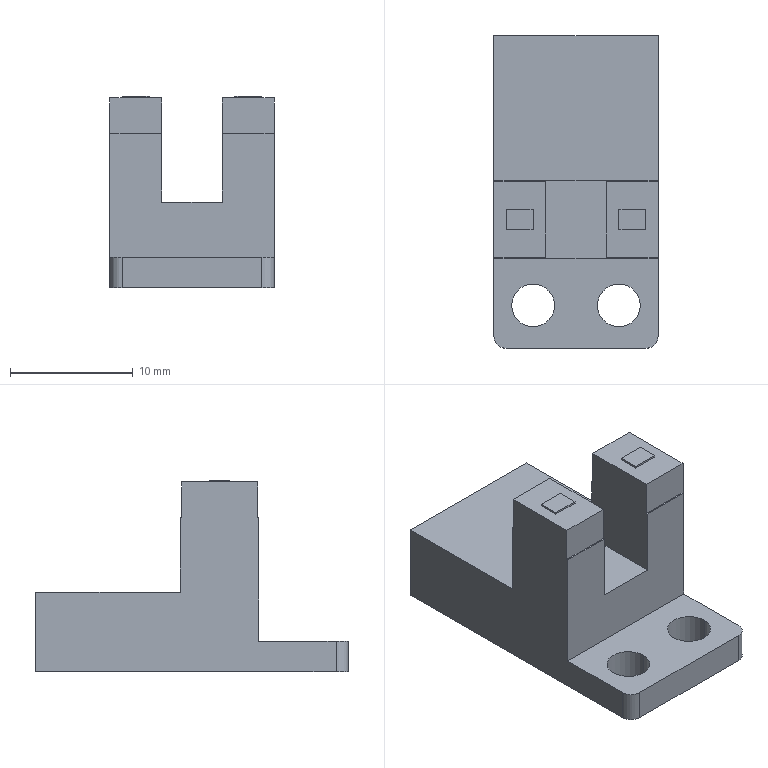Part | SolidWorks | features BaseBody 1 | 1 solid | 38 faces | box 13.4 x 25.5 x 15.65 mm | volume 2278 mm3 | plane 32 | cylinder 6 | commonest cylinder face diameters 3.5 x4 2 x2
STEP:
#1=CARTESIAN_POINT('',(304.797,206.806,-399.345));
#2=VERTEX_POINT('',#1);
#3=CARTESIAN_POINT('',(301.297,206.806,-399.345));
#4=VERTEX_POINT('',#3);
#5=CARTESIAN_POINT('',(303.047,206.806,-399.345));
#6=DIRECTION('',(0.,0.,-1.));
#7=DIRECTION('',(-1.,0.,0.));
#8=AXIS2_PLACEMENT_3D('',#5,#6,#7);
#9=CIRCLE('',#8,1.75);
#10=EDGE_CURVE('',#2,#4,#9,.T.);
#11=ORIENTED_EDGE('',*,*,#10,.F.);
#12=CARTESIAN_POINT('',(304.797,206.806,-401.845));
#13=VERTEX_POINT('',#12);
#14=CARTESIAN_POINT('',(304.797,206.806,-344.345));
#15=DIRECTION('',(0.,0.,-1.));
#16=VECTOR('',#15,1000.);
#17=LINE('',#14,#16);
#18=EDGE_CURVE('',#2,#13,#17,.T.);
#19=ORIENTED_EDGE('',*,*,#18,.T.);
#20=CARTESIAN_POINT('',(301.297,206.806,-401.845));
#21=VERTEX_POINT('',#20);
#22=CARTESIAN_POINT('',(303.047,206.806,-401.845));
#23=DIRECTION('',(0.,0.,-1.));
#24=DIRECTION('',(-1.,0.,0.));
#25=AXIS2_PLACEMENT_3D('',#22,#23,#24);
#26=CIRCLE('',#25,1.75);
#27=EDGE_CURVE('',#13,#21,#26,.T.);
#28=ORIENTED_EDGE('',*,*,#27,.T.);
#29=CARTESIAN_POINT('',(301.297,206.806,-344.345));
#30=DIRECTION('',(0.,0.,-1.));
#31=VECTOR('',#30,1000.);
#32=LINE('',#29,#31);
#33=EDGE_CURVE('',#4,#21,#32,.T.);
#34=ORIENTED_EDGE('',*,*,#33,.F.);
#35=EDGE_LOOP('',(#11,#19,#28,#34));
#36=FACE_OUTER_BOUND('',#35,.T.);
#37=CARTESIAN_POINT('',(303.047,206.806,-344.345));
#38=DIRECTION('',(0.,0.,-1.));
#39=DIRECTION('',(-1.,0.,0.));
#40=AXIS2_PLACEMENT_3D('',#37,#38,#39);
#41=CYLINDRICAL_SURFACE('',#40,1.75);
#42=ADVANCED_FACE('',(#36),#41,.F.);
#43=CARTESIAN_POINT('',(297.797,206.806,-399.345));
#44=VERTEX_POINT('',#43);
#45=CARTESIAN_POINT('',(294.297,206.806,-399.345));
#46=VERTEX_POINT('',#45);
#47=CARTESIAN_POINT('',(296.047,206.806,-399.345));
#48=DIRECTION('',(0.,0.,-1.));
#49=DIRECTION('',(-1.,0.,0.));
#50=AXIS2_PLACEMENT_3D('',#47,#48,#49);
#51=CIRCLE('',#50,1.75);
#52=EDGE_CURVE('',#44,#46,#51,.T.);
#53=ORIENTED_EDGE('',*,*,#52,.F.);
#54=CARTESIAN_POINT('',(297.797,206.806,-401.845));
#55=VERTEX_POINT('',#54);
#56=CARTESIAN_POINT('',(297.797,206.806,-344.345));
#57=DIRECTION('',(0.,0.,-1.));
#58=VECTOR('',#57,1000.);
#59=LINE('',#56,#58);
#60=EDGE_CURVE('',#44,#55,#59,.T.);
#61=ORIENTED_EDGE('',*,*,#60,.T.);
#62=CARTESIAN_POINT('',(294.297,206.806,-401.845));
#63=VERTEX_POINT('',#62);
#64=CARTESIAN_POINT('',(296.047,206.806,-401.845));
#65=DIRECTION('',(0.,0.,-1.));
#66=DIRECTION('',(-1.,0.,0.));
#67=AXIS2_PLACEMENT_3D('',#64,#65,#66);
#68=CIRCLE('',#67,1.75);
#69=EDGE_CURVE('',#55,#63,#68,.T.);
#70=ORIENTED_EDGE('',*,*,#69,.T.);
#71=CARTESIAN_POINT('',(294.297,206.806,-344.345));
#72=DIRECTION('',(0.,0.,-1.));
#73=VECTOR('',#72,1000.);
#74=LINE('',#71,#73);
#75=EDGE_CURVE('',#46,#63,#74,.T.);
#76=ORIENTED_EDGE('',*,*,#75,.F.);
#77=EDGE_LOOP('',(#53,#61,#70,#76));
#78=FACE_OUTER_BOUND('',#77,.T.);
#79=CARTESIAN_POINT('',(296.047,206.806,-344.345));
#80=DIRECTION('',(0.,0.,-1.));
#81=DIRECTION('',(-1.,0.,0.));
#82=AXIS2_PLACEMENT_3D('',#79,#80,#81);
#83=CYLINDRICAL_SURFACE('',#82,1.75);
#84=ADVANCED_FACE('',(#78),#83,.F.);
#85=CARTESIAN_POINT('',(303.047,206.806,-401.845));
#86=DIRECTION('',(0.,0.,-1.));
#87=DIRECTION('',(-1.,0.,0.));
#88=AXIS2_PLACEMENT_3D('',#85,#86,#87);
#89=CIRCLE('',#88,1.75);
#90=EDGE_CURVE('',#21,#13,#89,.T.);
#91=ORIENTED_EDGE('',*,*,#90,.F.);
#92=ORIENTED_EDGE('',*,*,#27,.F.);
#93=EDGE_LOOP('',(#91,#92));
#94=FACE_BOUND('',#93,.T.);
#95=CARTESIAN_POINT('',(296.047,206.806,-401.845));
#96=DIRECTION('',(0.,0.,-1.));
#97=DIRECTION('',(-1.,0.,0.));
#98=AXIS2_PLACEMENT_3D('',#95,#96,#97);
#99=CIRCLE('',#98,1.75);
#100=EDGE_CURVE('',#63,#55,#99,.T.);
#101=ORIENTED_EDGE('',*,*,#100,.F.);
#102=ORIENTED_EDGE('',*,*,#69,.F.);
#103=EDGE_LOOP('',(#101,#102));
#104=FACE_BOUND('',#103,.T.);
#105=CARTESIAN_POINT('',(292.847,228.806,-401.845));
#106=VERTEX_POINT('',#105);
#107=CARTESIAN_POINT('',(292.847,204.306,-401.845));
#108=VERTEX_POINT('',#107);
#109=CARTESIAN_POINT('',(292.847,228.806,-401.845));
#110=DIRECTION('',(0.,-1.,0.));
#111=VECTOR('',#110,1000.);
#112=LINE('',#109,#111);
#113=EDGE_CURVE('',#106,#108,#112,.T.);
#114=ORIENTED_EDGE('',*,*,#113,.F.);
#115=CARTESIAN_POINT('',(306.247,228.806,-401.845));
#116=VERTEX_POINT('',#115);
#117=CARTESIAN_POINT('',(306.247,228.806,-401.845));
#118=DIRECTION('',(-1.,0.,0.));
#119=VECTOR('',#118,1000.);
#120=LINE('',#117,#119);
#121=EDGE_CURVE('',#116,#106,#120,.T.);
#122=ORIENTED_EDGE('',*,*,#121,.F.);
#123=CARTESIAN_POINT('',(306.247,204.306,-401.845));
#124=VERTEX_POINT('',#123);
#125=CARTESIAN_POINT('',(306.247,228.806,-401.845));
#126=DIRECTION('',(0.,1.,0.));
#127=VECTOR('',#126,1000.);
#128=LINE('',#125,#127);
#129=EDGE_CURVE('',#124,#116,#128,.T.);
#130=ORIENTED_EDGE('',*,*,#129,.F.);
#131=CARTESIAN_POINT('',(305.247,203.306,-401.845));
#132=VERTEX_POINT('',#131);
#133=CARTESIAN_POINT('',(305.247,204.306,-401.845));
#134=DIRECTION('',(0.,0.,1.));
#135=DIRECTION('',(-1.,0.,0.));
#136=AXIS2_PLACEMENT_3D('',#133,#134,#135);
#137=CIRCLE('',#136,1.);
#138=EDGE_CURVE('',#132,#124,#137,.T.);
#139=ORIENTED_EDGE('',*,*,#138,.F.);
#140=CARTESIAN_POINT('',(293.847,203.306,-401.845));
#141=VERTEX_POINT('',#140);
#142=CARTESIAN_POINT('',(306.247,203.306,-401.845));
#143=DIRECTION('',(1.,0.,0.));
#144=VECTOR('',#143,1000.);
#145=LINE('',#142,#144);
#146=EDGE_CURVE('',#141,#132,#145,.T.);
#147=ORIENTED_EDGE('',*,*,#146,.F.);
#148=CARTESIAN_POINT('',(293.847,204.306,-401.845));
#149=DIRECTION('',(0.,0.,1.));
#150=DIRECTION('',(1.,0.,0.));
#151=AXIS2_PLACEMENT_3D('',#148,#149,#150);
#152=CIRCLE('',#151,1.);
#153=EDGE_CURVE('',#108,#141,#152,.T.);
#154=ORIENTED_EDGE('',*,*,#153,.F.);
#155=EDGE_LOOP('',(#114,#122,#130,#139,#147,#154));
#156=FACE_OUTER_BOUND('',#155,.T.);
#157=CARTESIAN_POINT('',(306.247,228.806,-401.845));
#158=DIRECTION('',(0.,0.,1.));
#159=DIRECTION('',(1.,0.,0.));
#160=AXIS2_PLACEMENT_3D('',#157,#158,#159);
#161=PLANE('',#160);
#162=ADVANCED_FACE('',(#94,#104,#156),#161,.F.);
#163=ORIENTED_EDGE('',*,*,#18,.F.);
#164=CARTESIAN_POINT('',(303.047,206.806,-399.345));
#165=DIRECTION('',(0.,0.,-1.));
#166=DIRECTION('',(-1.,0.,0.));
#167=AXIS2_PLACEMENT_3D('',#164,#165,#166);
#168=CIRCLE('',#167,1.75);
#169=EDGE_CURVE('',#4,#2,#168,.T.);
#170=ORIENTED_EDGE('',*,*,#169,.F.);
#171=ORIENTED_EDGE('',*,*,#33,.T.);
#172=ORIENTED_EDGE('',*,*,#90,.T.);
#173=EDGE_LOOP('',(#163,#170,#171,#172));
#174=FACE_OUTER_BOUND('',#173,.T.);
#175=CARTESIAN_POINT('',(303.047,206.806,-344.345));
#176=DIRECTION('',(0.,0.,-1.));
#177=DIRECTION('',(-1.,0.,0.));
#178=AXIS2_PLACEMENT_3D('',#175,#176,#177);
#179=CYLINDRICAL_SURFACE('',#178,1.75);
#180=ADVANCED_FACE('',(#174),#179,.F.);
#181=ORIENTED_EDGE('',*,*,#60,.F.);
#182=CARTESIAN_POINT('',(296.047,206.806,-399.345));
#183=DIRECTION('',(0.,0.,-1.));
#184=DIRECTION('',(-1.,0.,0.));
#185=AXIS2_PLACEMENT_3D('',#182,#183,#184);
#186=CIRCLE('',#185,1.75);
#187=EDGE_CURVE('',#46,#44,#186,.T.);
#188=ORIENTED_EDGE('',*,*,#187,.F.);
#189=ORIENTED_EDGE('',*,*,#75,.T.);
#190=ORIENTED_EDGE('',*,*,#100,.T.);
#191=EDGE_LOOP('',(#181,#188,#189,#190));
#192=FACE_OUTER_BOUND('',#191,.T.);
#193=CARTESIAN_POINT('',(296.047,206.806,-344.345));
#194=DIRECTION('',(0.,0.,-1.));
#195=DIRECTION('',(-1.,0.,0.));
#196=AXIS2_PLACEMENT_3D('',#193,#194,#195);
#197=CYLINDRICAL_SURFACE('',#196,1.75);
#198=ADVANCED_FACE('',(#192),#197,.F.);
#199=CARTESIAN_POINT('',(292.847,204.306,-399.345));
#200=VERTEX_POINT('',#199);
#201=CARTESIAN_POINT('',(292.847,204.306,-401.845));
#202=DIRECTION('',(0.,0.,-1.));
#203=VECTOR('',#202,1000.);
#204=LINE('',#201,#203);
#205=EDGE_CURVE('',#200,#108,#204,.T.);
#206=ORIENTED_EDGE('',*,*,#205,.T.);
#207=ORIENTED_EDGE('',*,*,#153,.T.);
#208=CARTESIAN_POINT('',(293.847,203.306,-399.345));
#209=VERTEX_POINT('',#208);
#210=CARTESIAN_POINT('',(293.847,203.306,-401.845));
#211=DIRECTION('',(0.,0.,1.));
#212=VECTOR('',#211,1000.);
#213=LINE('',#210,#212);
#214=EDGE_CURVE('',#141,#209,#213,.T.);
#215=ORIENTED_EDGE('',*,*,#214,.T.);
#216=CARTESIAN_POINT('',(293.847,204.306,-399.345));
#217=DIRECTION('',(0.,0.,-1.));
#218=DIRECTION('',(1.,0.,0.));
#219=AXIS2_PLACEMENT_3D('',#216,#217,#218);
#220=CIRCLE('',#219,1.);
#221=EDGE_CURVE('',#209,#200,#220,.T.);
#222=ORIENTED_EDGE('',*,*,#221,.T.);
#223=EDGE_LOOP('',(#206,#207,#215,#222));
#224=FACE_OUTER_BOUND('',#223,.T.);
#225=CARTESIAN_POINT('',(293.847,204.306,-401.845));
#226=DIRECTION('',(0.,0.,1.));
#227=DIRECTION('',(1.,0.,0.));
#228=AXIS2_PLACEMENT_3D('',#225,#226,#227);
#229=CYLINDRICAL_SURFACE('',#228,1.);
#230=ADVANCED_FACE('',(#224),#229,.T.);
#231=CARTESIAN_POINT('',(292.847,210.606,-399.345));
#232=VERTEX_POINT('',#231);
#233=CARTESIAN_POINT('',(292.847,228.806,-399.345));
#234=DIRECTION('',(0.,-1.,0.));
#235=VECTOR('',#234,1000.);
#236=LINE('',#233,#235);
#237=EDGE_CURVE('',#232,#200,#236,.T.);
#238=ORIENTED_EDGE('',*,*,#237,.F.);
#239=CARTESIAN_POINT('',(292.847,210.606,-389.245));
#240=VERTEX_POINT('',#239);
#241=CARTESIAN_POINT('',(292.847,210.606,-401.845));
#242=DIRECTION('',(0.,0.,-1.));
#243=VECTOR('',#242,1000.);
#244=LINE('',#241,#243);
#245=EDGE_CURVE('',#240,#232,#244,.T.);
#246=ORIENTED_EDGE('',*,*,#245,.F.);
#247=CARTESIAN_POINT('',(292.847,210.706,-389.245));
#248=VERTEX_POINT('',#247);
#249=CARTESIAN_POINT('',(292.847,228.806,-389.245));
#250=DIRECTION('',(0.,-1.,0.));
#251=VECTOR('',#250,1000.);
#252=LINE('',#249,#251);
#253=EDGE_CURVE('',#248,#240,#252,.T.);
#254=ORIENTED_EDGE('',*,*,#253,.F.);
#255=CARTESIAN_POINT('',(292.847,210.706,-386.345));
#256=VERTEX_POINT('',#255);
#257=CARTESIAN_POINT('',(292.847,210.706,-401.845));
#258=DIRECTION('',(0.,0.,-1.));
#259=VECTOR('',#258,1000.);
#260=LINE('',#257,#259);
#261=EDGE_CURVE('',#256,#248,#260,.T.);
#262=ORIENTED_EDGE('',*,*,#261,.F.);
#263=CARTESIAN_POINT('',(292.847,216.906,-386.345));
#264=VERTEX_POINT('',#263);
#265=CARTESIAN_POINT('',(292.847,228.806,-386.345));
#266=DIRECTION('',(0.,-1.,0.));
#267=VECTOR('',#266,1000.);
#268=LINE('',#265,#267);
#269=EDGE_CURVE('',#264,#256,#268,.T.);
#270=ORIENTED_EDGE('',*,*,#269,.F.);
#271=CARTESIAN_POINT('',(292.847,216.906,-389.245));
#272=VERTEX_POINT('',#271);
#273=CARTESIAN_POINT('',(292.847,216.906,-401.845));
#274=DIRECTION('',(0.,0.,1.));
#275=VECTOR('',#274,1000.);
#276=LINE('',#273,#275);
#277=EDGE_CURVE('',#272,#264,#276,.T.);
#278=ORIENTED_EDGE('',*,*,#277,.F.);
#279=CARTESIAN_POINT('',(292.847,217.006,-389.245));
#280=VERTEX_POINT('',#279);
#281=CARTESIAN_POINT('',(292.847,228.806,-389.245));
#282=DIRECTION('',(0.,-1.,0.));
#283=VECTOR('',#282,1000.);
#284=LINE('',#281,#283);
#285=EDGE_CURVE('',#280,#272,#284,.T.);
#286=ORIENTED_EDGE('',*,*,#285,.F.);
#287=CARTESIAN_POINT('',(292.847,217.006,-395.345));
#288=VERTEX_POINT('',#287);
#289=CARTESIAN_POINT('',(292.847,217.006,-401.845));
#290=DIRECTION('',(0.,0.,1.));
#291=VECTOR('',#290,1000.);
#292=LINE('',#289,#291);
#293=EDGE_CURVE('',#288,#280,#292,.T.);
#294=ORIENTED_EDGE('',*,*,#293,.F.);
#295=CARTESIAN_POINT('',(292.847,228.806,-395.345));
#296=VERTEX_POINT('',#295);
#297=CARTESIAN_POINT('',(292.847,228.806,-395.345));
#298=DIRECTION('',(0.,-1.,0.));
#299=VECTOR('',#298,1000.);
#300=LINE('',#297,#299);
#301=EDGE_CURVE('',#296,#288,#300,.T.);
#302=ORIENTED_EDGE('',*,*,#301,.F.);
#303=CARTESIAN_POINT('',(292.847,228.806,-401.845));
#304=DIRECTION('',(0.,0.,1.));
#305=VECTOR('',#304,1000.);
#306=LINE('',#303,#305);
#307=EDGE_CURVE('',#106,#296,#306,.T.);
#308=ORIENTED_EDGE('',*,*,#307,.F.);
#309=ORIENTED_EDGE('',*,*,#113,.T.);
#310=ORIENTED_EDGE('',*,*,#205,.F.);
#311=EDGE_LOOP('',(#238,#246,#254,#262,#270,#278,#286,#294,#302,#308,#309,#310));
#312=FACE_OUTER_BOUND('',#311,.T.);
#313=CARTESIAN_POINT('',(292.847,228.806,-401.845));
#314=DIRECTION('',(1.,0.,0.));
#315=DIRECTION('',(0.,0.,-1.));
#316=AXIS2_PLACEMENT_3D('',#313,#314,#315);
#317=PLANE('',#316);
#318=ADVANCED_FACE('',(#312),#317,.F.);
#319=ORIENTED_EDGE('',*,*,#307,.T.);
#320=CARTESIAN_POINT('',(306.247,228.806,-395.345));
#321=VERTEX_POINT('',#320);
#322=CARTESIAN_POINT('',(357.247,228.806,-395.345));
#323=DIRECTION('',(1.,0.,0.));
#324=VECTOR('',#323,1000.);
#325=LINE('',#322,#324);
#326=EDGE_CURVE('',#296,#321,#325,.T.);
#327=ORIENTED_EDGE('',*,*,#326,.T.);
#328=CARTESIAN_POINT('',(306.247,228.806,-444.345));
#329=DIRECTION('',(0.,0.,-1.));
#330=VECTOR('',#329,1000.);
#331=LINE('',#328,#330);
#332=EDGE_CURVE('',#321,#116,#331,.T.);
#333=ORIENTED_EDGE('',*,*,#332,.T.);
#334=ORIENTED_EDGE('',*,*,#121,.T.);
#335=EDGE_LOOP('',(#319,#327,#333,#334));
#336=FACE_OUTER_BOUND('',#335,.T.);
#337=CARTESIAN_POINT('',(357.247,228.806,-444.345));
#338=DIRECTION('',(0.,1.,0.));
#339=DIRECTION('',(0.,0.,1.));
#340=AXIS2_PLACEMENT_3D('',#337,#338,#339);
#341=PLANE('',#340);
#342=ADVANCED_FACE('',(#336),#341,.T.);
#343=ORIENTED_EDGE('',*,*,#129,.T.);
#344=ORIENTED_EDGE('',*,*,#332,.F.);
#345=CARTESIAN_POINT('',(306.247,217.006,-395.345));
#346=VERTEX_POINT('',#345);
#347=CARTESIAN_POINT('',(306.247,228.806,-395.345));
#348=DIRECTION('',(0.,1.,0.));
#349=VECTOR('',#348,1000.);
#350=LINE('',#347,#349);
#351=EDGE_CURVE('',#346,#321,#350,.T.);
#352=ORIENTED_EDGE('',*,*,#351,.F.);
#353=CARTESIAN_POINT('',(306.247,217.006,-389.245));
#354=VERTEX_POINT('',#353);
#355=CARTESIAN_POINT('',(306.247,217.006,-386.345));
#356=DIRECTION('',(0.,0.,-1.));
#357=VECTOR('',#356,1000.);
#358=LINE('',#355,#357);
#359=EDGE_CURVE('',#354,#346,#358,.T.);
#360=ORIENTED_EDGE('',*,*,#359,.F.);
#361=CARTESIAN_POINT('',(306.247,216.906,-389.245));
#362=VERTEX_POINT('',#361);
#363=CARTESIAN_POINT('',(306.247,228.806,-389.245));
#364=DIRECTION('',(0.,1.,0.));
#365=VECTOR('',#364,1000.);
#366=LINE('',#363,#365);
#367=EDGE_CURVE('',#362,#354,#366,.T.);
#368=ORIENTED_EDGE('',*,*,#367,.F.);
#369=CARTESIAN_POINT('',(306.247,216.906,-386.345));
#370=VERTEX_POINT('',#369);
#371=CARTESIAN_POINT('',(306.247,216.906,-386.345));
#372=DIRECTION('',(0.,0.,-1.));
#373=VECTOR('',#372,1000.);
#374=LINE('',#371,#373);
#375=EDGE_CURVE('',#370,#362,#374,.T.);
#376=ORIENTED_EDGE('',*,*,#375,.F.);
#377=CARTESIAN_POINT('',(306.247,210.706,-386.345));
#378=VERTEX_POINT('',#377);
#379=CARTESIAN_POINT('',(306.247,228.806,-386.345));
#380=DIRECTION('',(0.,1.,0.));
#381=VECTOR('',#380,1000.);
#382=LINE('',#379,#381);
#383=EDGE_CURVE('',#378,#370,#382,.T.);
#384=ORIENTED_EDGE('',*,*,#383,.F.);
#385=CARTESIAN_POINT('',(306.247,210.706,-389.245));
#386=VERTEX_POINT('',#385);
#387=CARTESIAN_POINT('',(306.247,210.706,-386.345));
#388=DIRECTION('',(0.,0.,1.));
#389=VECTOR('',#388,1000.);
#390=LINE('',#387,#389);
#391=EDGE_CURVE('',#386,#378,#390,.T.);
#392=ORIENTED_EDGE('',*,*,#391,.F.);
#393=CARTESIAN_POINT('',(306.247,210.606,-389.245));
#394=VERTEX_POINT('',#393);
#395=CARTESIAN_POINT('',(306.247,228.806,-389.245));
#396=DIRECTION('',(0.,1.,0.));
#397=VECTOR('',#396,1000.);
#398=LINE('',#395,#397);
#399=EDGE_CURVE('',#394,#386,#398,.T.);
#400=ORIENTED_EDGE('',*,*,#399,.F.);
#401=CARTESIAN_POINT('',(306.247,210.606,-399.345));
#402=VERTEX_POINT('',#401);
#403=CARTESIAN_POINT('',(306.247,210.606,-386.345));
#404=DIRECTION('',(0.,0.,1.));
#405=VECTOR('',#404,1000.);
#406=LINE('',#403,#405);
#407=EDGE_CURVE('',#402,#394,#406,.T.);
#408=ORIENTED_EDGE('',*,*,#407,.F.);
#409=CARTESIAN_POINT('',(306.247,204.306,-399.345));
#410=VERTEX_POINT('',#409);
#411=CARTESIAN_POINT('',(306.247,228.806,-399.345));
#412=DIRECTION('',(0.,1.,0.));
#413=VECTOR('',#412,1000.);
#414=LINE('',#411,#413);
#415=EDGE_CURVE('',#410,#402,#414,.T.);
#416=ORIENTED_EDGE('',*,*,#415,.F.);
#417=CARTESIAN_POINT('',(306.247,204.306,-386.345));
#418=DIRECTION('',(0.,0.,1.));
#419=VECTOR('',#418,1000.);
#420=LINE('',#417,#419);
#421=EDGE_CURVE('',#124,#410,#420,.T.);
#422=ORIENTED_EDGE('',*,*,#421,.F.);
#423=EDGE_LOOP('',(#343,#344,#352,#360,#368,#376,#384,#392,#400,#408,#416,#422));
#424=FACE_OUTER_BOUND('',#423,.T.);
#425=CARTESIAN_POINT('',(306.247,228.806,-386.345));
#426=DIRECTION('',(-1.,0.,0.));
#427=DIRECTION('',(0.,0.,1.));
#428=AXIS2_PLACEMENT_3D('',#425,#426,#427);
#429=PLANE('',#428);
#430=ADVANCED_FACE('',(#424),#429,.F.);
#431=ORIENTED_EDGE('',*,*,#421,.T.);
#432=CARTESIAN_POINT('',(305.247,203.306,-399.345));
#433=VERTEX_POINT('',#432);
#434=CARTESIAN_POINT('',(305.247,204.306,-399.345));
#435=DIRECTION('',(0.,0.,-1.));
#436=DIRECTION('',(-1.,0.,0.));
#437=AXIS2_PLACEMENT_3D('',#434,#435,#436);
#438=CIRCLE('',#437,1.);
#439=EDGE_CURVE('',#410,#433,#438,.T.);
#440=ORIENTED_EDGE('',*,*,#439,.T.);
#441=CARTESIAN_POINT('',(305.247,203.306,-386.345));
#442=DIRECTION('',(0.,0.,-1.));
#443=VECTOR('',#442,1000.);
#444=LINE('',#441,#443);
#445=EDGE_CURVE('',#433,#132,#444,.T.);
#446=ORIENTED_EDGE('',*,*,#445,.T.);
#447=ORIENTED_EDGE('',*,*,#138,.T.);
#448=EDGE_LOOP('',(#431,#440,#446,#447));
#449=FACE_OUTER_BOUND('',#448,.T.);
#450=CARTESIAN_POINT('',(305.247,204.306,-386.345));
#451=DIRECTION('',(0.,0.,-1.));
#452=DIRECTION('',(-1.,0.,0.));
#453=AXIS2_PLACEMENT_3D('',#450,#451,#452);
#454=CYLINDRICAL_SURFACE('',#453,1.);
#455=ADVANCED_FACE('',(#449),#454,.T.);
#456=ORIENTED_EDGE('',*,*,#146,.T.);
#457=ORIENTED_EDGE('',*,*,#445,.F.);
#458=CARTESIAN_POINT('',(357.247,203.306,-399.345));
#459=DIRECTION('',(1.,0.,0.));
#460=VECTOR('',#459,1000.);
#461=LINE('',#458,#460);
#462=EDGE_CURVE('',#209,#433,#461,.T.);
#463=ORIENTED_EDGE('',*,*,#462,.F.);
#464=ORIENTED_EDGE('',*,*,#214,.F.);
#465=EDGE_LOOP('',(#456,#457,#463,#464));
#466=FACE_OUTER_BOUND('',#465,.T.);
#467=CARTESIAN_POINT('',(357.247,203.306,-444.345));
#468=DIRECTION('',(0.,1.,0.));
#469=DIRECTION('',(0.,0.,1.));
#470=AXIS2_PLACEMENT_3D('',#467,#468,#469);
#471=PLANE('',#470);
#472=ADVANCED_FACE('',(#466),#471,.F.);
#473=ORIENTED_EDGE('',*,*,#169,.T.);
#474=ORIENTED_EDGE('',*,*,#10,.T.);
#475=EDGE_LOOP('',(#473,#474));
#476=FACE_BOUND('',#475,.T.);
#477=ORIENTED_EDGE('',*,*,#187,.T.);
#478=ORIENTED_EDGE('',*,*,#52,.T.);
#479=EDGE_LOOP('',(#477,#478));
#480=FACE_BOUND('',#479,.T.);
#481=ORIENTED_EDGE('',*,*,#462,.T.);
#482=ORIENTED_EDGE('',*,*,#439,.F.);
#483=ORIENTED_EDGE('',*,*,#415,.T.);
#484=CARTESIAN_POINT('',(257.247,210.606,-399.345));
#485=DIRECTION('',(1.,0.,0.));
#486=VECTOR('',#485,1000.);
#487=LINE('',#484,#486);
#488=EDGE_CURVE('',#232,#402,#487,.T.);
#489=ORIENTED_EDGE('',*,*,#488,.F.);
#490=ORIENTED_EDGE('',*,*,#237,.T.);
#491=ORIENTED_EDGE('',*,*,#221,.F.);
#492=EDGE_LOOP('',(#481,#482,#483,#489,#490,#491));
#493=FACE_OUTER_BOUND('',#492,.T.);
#494=CARTESIAN_POINT('',(257.247,203.306,-399.345));
#495=DIRECTION('',(0.,0.,-1.));
#496=DIRECTION('',(-1.,0.,0.));
#497=AXIS2_PLACEMENT_3D('',#494,#495,#496);
#498=PLANE('',#497);
#499=ADVANCED_FACE('',(#476,#480,#493),#498,.F.);
#500=CARTESIAN_POINT('',(297.063,210.606,-394.845));
#501=VERTEX_POINT('',#500);
#502=CARTESIAN_POINT('',(302.031,210.606,-394.845));
#503=VERTEX_POINT('',#502);
#504=CARTESIAN_POINT('',(257.247,210.606,-394.845));
#505=DIRECTION('',(1.,0.,0.));
#506=VECTOR('',#505,1000.);
#507=LINE('',#504,#506);
#508=EDGE_CURVE('',#501,#503,#507,.T.);
#509=ORIENTED_EDGE('',*,*,#508,.F.);
#510=CARTESIAN_POINT('',(297.063,210.606,-389.245));
#511=VERTEX_POINT('',#510);
#512=CARTESIAN_POINT('',(297.063,210.606,-399.345));
#513=DIRECTION('',(0.,0.,-1.));
#514=VECTOR('',#513,1000.);
#515=LINE('',#512,#514);
#516=EDGE_CURVE('',#511,#501,#515,.T.);
#517=ORIENTED_EDGE('',*,*,#516,.F.);
#518=CARTESIAN_POINT('',(257.247,210.606,-389.245));
#519=DIRECTION('',(1.,0.,0.));
#520=VECTOR('',#519,1000.);
#521=LINE('',#518,#520);
#522=EDGE_CURVE('',#240,#511,#521,.T.);
#523=ORIENTED_EDGE('',*,*,#522,.F.);
#524=ORIENTED_EDGE('',*,*,#245,.T.);
#525=ORIENTED_EDGE('',*,*,#488,.T.);
#526=ORIENTED_EDGE('',*,*,#407,.T.);
#527=CARTESIAN_POINT('',(302.031,210.606,-389.245));
#528=VERTEX_POINT('',#527);
#529=CARTESIAN_POINT('',(257.247,210.606,-389.245));
#530=DIRECTION('',(1.,0.,0.));
#531=VECTOR('',#530,1000.);
#532=LINE('',#529,#531);
#533=EDGE_CURVE('',#528,#394,#532,.T.);
#534=ORIENTED_EDGE('',*,*,#533,.F.);
#535=CARTESIAN_POINT('',(302.031,210.606,-399.345));
#536=DIRECTION('',(0.,0.,1.));
#537=VECTOR('',#536,1000.);
#538=LINE('',#535,#537);
#539=EDGE_CURVE('',#503,#528,#538,.T.);
#540=ORIENTED_EDGE('',*,*,#539,.F.);
#541=EDGE_LOOP('',(#509,#517,#523,#524,#525,#526,#534,#540));
#542=FACE_OUTER_BOUND('',#541,.T.);
#543=CARTESIAN_POINT('',(257.247,210.606,-399.345));
#544=DIRECTION('',(0.,1.,0.));
#545=DIRECTION('',(0.,0.,1.));
#546=AXIS2_PLACEMENT_3D('',#543,#544,#545);
#547=PLANE('',#546);
#548=ADVANCED_FACE('',(#542),#547,.F.);
#549=CARTESIAN_POINT('',(297.063,210.706,-389.245));
#550=VERTEX_POINT('',#549);
#551=CARTESIAN_POINT('',(257.247,210.706,-389.245));
#552=DIRECTION('',(1.,0.,0.));
#553=VECTOR('',#552,1000.);
#554=LINE('',#551,#553);
#555=EDGE_CURVE('',#248,#550,#554,.T.);
#556=ORIENTED_EDGE('',*,*,#555,.F.);
#557=ORIENTED_EDGE('',*,*,#253,.T.);
#558=ORIENTED_EDGE('',*,*,#522,.T.);
#559=CARTESIAN_POINT('',(297.063,210.606,-389.245));
#560=DIRECTION('',(0.,-1.,0.));
#561=VECTOR('',#560,1000.);
#562=LINE('',#559,#561);
#563=EDGE_CURVE('',#550,#511,#562,.T.);
#564=ORIENTED_EDGE('',*,*,#563,.F.);
#565=EDGE_LOOP('',(#556,#557,#558,#564));
#566=FACE_OUTER_BOUND('',#565,.T.);
#567=CARTESIAN_POINT('',(257.247,210.606,-389.245));
#568=DIRECTION('',(0.,0.,-1.));
#569=DIRECTION('',(-1.,0.,0.));
#570=AXIS2_PLACEMENT_3D('',#567,#568,#569);
#571=PLANE('',#570);
#572=ADVANCED_FACE('',(#566),#571,.F.);
#573=CARTESIAN_POINT('',(297.063,210.706,-386.345));
#574=VERTEX_POINT('',#573);
#575=CARTESIAN_POINT('',(257.247,210.706,-386.345));
#576=DIRECTION('',(1.,0.,0.));
#577=VECTOR('',#576,1000.);
#578=LINE('',#575,#577);
#579=EDGE_CURVE('',#256,#574,#578,.T.);
#580=ORIENTED_EDGE('',*,*,#579,.F.);
#581=ORIENTED_EDGE('',*,*,#261,.T.);
#582=ORIENTED_EDGE('',*,*,#555,.T.);
#583=CARTESIAN_POINT('',(297.063,210.706,-389.245));
#584=DIRECTION('',(0.,0.,-1.));
#585=VECTOR('',#584,1000.);
#586=LINE('',#583,#585);
#587=EDGE_CURVE('',#574,#550,#586,.T.);
#588=ORIENTED_EDGE('',*,*,#587,.F.);
#589=EDGE_LOOP('',(#580,#581,#582,#588));
#590=FACE_OUTER_BOUND('',#589,.T.);
#591=CARTESIAN_POINT('',(257.247,210.706,-389.245));
#592=DIRECTION('',(0.,1.,0.));
#593=DIRECTION('',(0.,0.,1.));
#594=AXIS2_PLACEMENT_3D('',#591,#592,#593);
#595=PLANE('',#594);
#596=ADVANCED_FACE('',(#590),#595,.F.);
#597=CARTESIAN_POINT('',(296.047,214.646,-386.345));
#598=VERTEX_POINT('',#597);
#599=CARTESIAN_POINT('',(293.847,214.646,-386.345));
#600=VERTEX_POINT('',#599);
#601=CARTESIAN_POINT('',(296.047,214.646,-386.345));
#602=DIRECTION('',(-1.,0.,0.));
#603=VECTOR('',#602,1000.);
#604=LINE('',#601,#603);
#605=EDGE_CURVE('',#598,#600,#604,.T.);
#606=ORIENTED_EDGE('',*,*,#605,.F.);
#607=CARTESIAN_POINT('',(296.047,212.966,-386.345));
#608=VERTEX_POINT('',#607);
#609=CARTESIAN_POINT('',(296.047,228.806,-386.345));
#610=DIRECTION('',(0.,1.,0.));
#611=VECTOR('',#610,1000.);
#612=LINE('',#609,#611);
#613=EDGE_CURVE('',#608,#598,#612,.T.);
#614=ORIENTED_EDGE('',*,*,#613,.F.);
#615=CARTESIAN_POINT('',(293.847,212.966,-386.345));
#616=VERTEX_POINT('',#615);
#617=CARTESIAN_POINT('',(296.047,212.966,-386.345));
#618=DIRECTION('',(1.,0.,0.));
#619=VECTOR('',#618,1000.);
#620=LINE('',#617,#619);
#621=EDGE_CURVE('',#616,#608,#620,.T.);
#622=ORIENTED_EDGE('',*,*,#621,.F.);
#623=CARTESIAN_POINT('',(293.847,228.806,-386.345));
#624=DIRECTION('',(0.,-1.,0.));
#625=VECTOR('',#624,1000.);
#626=LINE('',#623,#625);
#627=EDGE_CURVE('',#600,#616,#626,.T.);
#628=ORIENTED_EDGE('',*,*,#627,.F.);
#629=EDGE_LOOP('',(#606,#614,#622,#628));
#630=FACE_BOUND('',#629,.T.);
#631=CARTESIAN_POINT('',(297.063,216.906,-386.345));
#632=VERTEX_POINT('',#631);
#633=CARTESIAN_POINT('',(297.063,228.806,-386.345));
#634=DIRECTION('',(0.,-1.,0.));
#635=VECTOR('',#634,1000.);
#636=LINE('',#633,#635);
#637=EDGE_CURVE('',#632,#574,#636,.T.);
#638=ORIENTED_EDGE('',*,*,#637,.F.);
#639=CARTESIAN_POINT('',(296.047,216.906,-386.345));
#640=DIRECTION('',(1.,0.,0.));
#641=VECTOR('',#640,1000.);
#642=LINE('',#639,#641);
#643=EDGE_CURVE('',#264,#632,#642,.T.);
#644=ORIENTED_EDGE('',*,*,#643,.F.);
#645=ORIENTED_EDGE('',*,*,#269,.T.);
#646=ORIENTED_EDGE('',*,*,#579,.T.);
#647=EDGE_LOOP('',(#638,#644,#645,#646));
#648=FACE_OUTER_BOUND('',#647,.T.);
#649=CARTESIAN_POINT('',(296.047,228.806,-386.345));
#650=DIRECTION('',(0.,0.,-1.));
#651=DIRECTION('',(-1.,0.,0.));
#652=AXIS2_PLACEMENT_3D('',#649,#650,#651);
#653=PLANE('',#652);
#654=ADVANCED_FACE('',(#630,#648),#653,.F.);
#655=CARTESIAN_POINT('',(297.063,216.906,-389.245));
#656=VERTEX_POINT('',#655);
#657=CARTESIAN_POINT('',(297.063,216.906,-386.345));
#658=DIRECTION('',(0.,0.,1.));
#659=VECTOR('',#658,1000.);
#660=LINE('',#657,#659);
#661=EDGE_CURVE('',#656,#632,#660,.T.);
#662=ORIENTED_EDGE('',*,*,#661,.F.);
#663=CARTESIAN_POINT('',(257.247,216.906,-389.245));
#664=DIRECTION('',(1.,0.,0.));
#665=VECTOR('',#664,1000.);
#666=LINE('',#663,#665);
#667=EDGE_CURVE('',#272,#656,#666,.T.);
#668=ORIENTED_EDGE('',*,*,#667,.F.);
#669=ORIENTED_EDGE('',*,*,#277,.T.);
#670=ORIENTED_EDGE('',*,*,#643,.T.);
#671=EDGE_LOOP('',(#662,#668,#669,#670));
#672=FACE_OUTER_BOUND('',#671,.T.);
#673=CARTESIAN_POINT('',(257.247,216.906,-386.345));
#674=DIRECTION('',(0.,-1.,0.));
#675=DIRECTION('',(0.,0.,-1.));
#676=AXIS2_PLACEMENT_3D('',#673,#674,#675);
#677=PLANE('',#676);
#678=ADVANCED_FACE('',(#672),#677,.F.);
#679=CARTESIAN_POINT('',(297.063,217.006,-389.245));
#680=VERTEX_POINT('',#679);
#681=CARTESIAN_POINT('',(257.247,217.006,-389.245));
#682=DIRECTION('',(1.,0.,0.));
#683=VECTOR('',#682,1000.);
#684=LINE('',#681,#683);
#685=EDGE_CURVE('',#280,#680,#684,.T.);
#686=ORIENTED_EDGE('',*,*,#685,.F.);
#687=ORIENTED_EDGE('',*,*,#285,.T.);
#688=ORIENTED_EDGE('',*,*,#667,.T.);
#689=CARTESIAN_POINT('',(297.063,216.906,-389.245));
#690=DIRECTION('',(0.,-1.,0.));
#691=VECTOR('',#690,1000.);
#692=LINE('',#689,#691);
#693=EDGE_CURVE('',#680,#656,#692,.T.);
#694=ORIENTED_EDGE('',*,*,#693,.F.);
#695=EDGE_LOOP('',(#686,#687,#688,#694));
#696=FACE_OUTER_BOUND('',#695,.T.);
#697=CARTESIAN_POINT('',(257.247,216.906,-389.245));
#698=DIRECTION('',(0.,0.,-1.));
#699=DIRECTION('',(-1.,0.,0.));
#700=AXIS2_PLACEMENT_3D('',#697,#698,#699);
#701=PLANE('',#700);
#702=ADVANCED_FACE('',(#696),#701,.F.);
#703=ORIENTED_EDGE('',*,*,#685,.T.);
#704=CARTESIAN_POINT('',(297.063,217.006,-394.845));
#705=VERTEX_POINT('',#704);
#706=CARTESIAN_POINT('',(297.063,217.006,-389.245));
#707=DIRECTION('',(0.,0.,1.));
#708=VECTOR('',#707,1000.);
#709=LINE('',#706,#708);
#710=EDGE_CURVE('',#705,#680,#709,.T.);
#711=ORIENTED_EDGE('',*,*,#710,.F.);
#712=CARTESIAN_POINT('',(302.031,217.006,-394.845));
#713=VERTEX_POINT('',#712);
#714=CARTESIAN_POINT('',(257.247,217.006,-394.845));
#715=DIRECTION('',(-1.,0.,0.));
#716=VECTOR('',#715,1000.);
#717=LINE('',#714,#716);
#718=EDGE_CURVE('',#713,#705,#717,.T.);
#719=ORIENTED_EDGE('',*,*,#718,.F.);
#720=CARTESIAN_POINT('',(302.031,217.006,-389.245));
#721=VERTEX_POINT('',#720);
#722=CARTESIAN_POINT('',(302.031,217.006,-389.245));
#723=DIRECTION('',(0.,0.,-1.));
#724=VECTOR('',#723,1000.);
#725=LINE('',#722,#724);
#726=EDGE_CURVE('',#721,#713,#725,.T.);
#727=ORIENTED_EDGE('',*,*,#726,.F.);
#728=CARTESIAN_POINT('',(257.247,217.006,-389.245));
#729=DIRECTION('',(-1.,0.,0.));
#730=VECTOR('',#729,1000.);
#731=LINE('',#728,#730);
#732=EDGE_CURVE('',#354,#721,#731,.T.);
#733=ORIENTED_EDGE('',*,*,#732,.F.);
#734=ORIENTED_EDGE('',*,*,#359,.T.);
#735=CARTESIAN_POINT('',(257.247,217.006,-395.345));
#736=DIRECTION('',(1.,0.,0.));
#737=VECTOR('',#736,1000.);
#738=LINE('',#735,#737);
#739=EDGE_CURVE('',#288,#346,#738,.T.);
#740=ORIENTED_EDGE('',*,*,#739,.F.);
#741=ORIENTED_EDGE('',*,*,#293,.T.);
#742=EDGE_LOOP('',(#703,#711,#719,#727,#733,#734,#740,#741));
#743=FACE_OUTER_BOUND('',#742,.T.);
#744=CARTESIAN_POINT('',(257.247,217.006,-389.245));
#745=DIRECTION('',(0.,-1.,0.));
#746=DIRECTION('',(0.,0.,-1.));
#747=AXIS2_PLACEMENT_3D('',#744,#745,#746);
#748=PLANE('',#747);
#749=ADVANCED_FACE('',(#743),#748,.F.);
#750=ORIENTED_EDGE('',*,*,#739,.T.);
#751=ORIENTED_EDGE('',*,*,#351,.T.);
#752=ORIENTED_EDGE('',*,*,#326,.F.);
#753=ORIENTED_EDGE('',*,*,#301,.T.);
#754=EDGE_LOOP('',(#750,#751,#752,#753));
#755=FACE_OUTER_BOUND('',#754,.T.);
#756=CARTESIAN_POINT('',(257.247,217.006,-395.345));
#757=DIRECTION('',(0.,0.,-1.));
#758=DIRECTION('',(-1.,0.,0.));
#759=AXIS2_PLACEMENT_3D('',#756,#757,#758);
#760=PLANE('',#759);
#761=ADVANCED_FACE('',(#755),#760,.F.);
#762=CARTESIAN_POINT('',(302.031,216.906,-389.245));
#763=VERTEX_POINT('',#762);
#764=CARTESIAN_POINT('',(257.247,216.906,-389.245));
#765=DIRECTION('',(-1.,0.,0.));
#766=VECTOR('',#765,1000.);
#767=LINE('',#764,#766);
#768=EDGE_CURVE('',#362,#763,#767,.T.);
#769=ORIENTED_EDGE('',*,*,#768,.F.);
#770=ORIENTED_EDGE('',*,*,#367,.T.);
#771=ORIENTED_EDGE('',*,*,#732,.T.);
#772=CARTESIAN_POINT('',(302.031,216.906,-389.245));
#773=DIRECTION('',(0.,1.,0.));
#774=VECTOR('',#773,1000.);
#775=LINE('',#772,#774);
#776=EDGE_CURVE('',#763,#721,#775,.T.);
#777=ORIENTED_EDGE('',*,*,#776,.F.);
#778=EDGE_LOOP('',(#769,#770,#771,#777));
#779=FACE_OUTER_BOUND('',#778,.T.);
#780=CARTESIAN_POINT('',(257.247,216.906,-389.245));
#781=DIRECTION('',(0.,0.,-1.));
#782=DIRECTION('',(-1.,0.,0.));
#783=AXIS2_PLACEMENT_3D('',#780,#781,#782);
#784=PLANE('',#783);
#785=ADVANCED_FACE('',(#779),#784,.F.);
#786=CARTESIAN_POINT('',(302.031,216.906,-386.345));
#787=VERTEX_POINT('',#786);
#788=CARTESIAN_POINT('',(257.247,216.906,-386.345));
#789=DIRECTION('',(-1.,0.,0.));
#790=VECTOR('',#789,1000.);
#791=LINE('',#788,#790);
#792=EDGE_CURVE('',#370,#787,#791,.T.);
#793=ORIENTED_EDGE('',*,*,#792,.F.);
#794=ORIENTED_EDGE('',*,*,#375,.T.);
#795=ORIENTED_EDGE('',*,*,#768,.T.);
#796=CARTESIAN_POINT('',(302.031,216.906,-386.345));
#797=DIRECTION('',(0.,0.,-1.));
#798=VECTOR('',#797,1000.);
#799=LINE('',#796,#798);
#800=EDGE_CURVE('',#787,#763,#799,.T.);
#801=ORIENTED_EDGE('',*,*,#800,.F.);
#802=EDGE_LOOP('',(#793,#794,#795,#801));
#803=FACE_OUTER_BOUND('',#802,.T.);
#804=CARTESIAN_POINT('',(257.247,216.906,-386.345));
#805=DIRECTION('',(0.,-1.,0.));
#806=DIRECTION('',(0.,0.,-1.));
#807=AXIS2_PLACEMENT_3D('',#804,#805,#806);
#808=PLANE('',#807);
#809=ADVANCED_FACE('',(#803),#808,.F.);
#810=CARTESIAN_POINT('',(303.047,214.646,-386.345));
#811=VERTEX_POINT('',#810);
#812=CARTESIAN_POINT('',(303.047,212.966,-386.345));
#813=VERTEX_POINT('',#812);
#814=CARTESIAN_POINT('',(303.047,228.806,-386.345));
#815=DIRECTION('',(0.,-1.,0.));
#816=VECTOR('',#815,1000.);
#817=LINE('',#814,#816);
#818=EDGE_CURVE('',#811,#813,#817,.T.);
#819=ORIENTED_EDGE('',*,*,#818,.F.);
#820=CARTESIAN_POINT('',(305.247,214.646,-386.345));
#821=VERTEX_POINT('',#820);
#822=CARTESIAN_POINT('',(302.031,214.646,-386.345));
#823=DIRECTION('',(-1.,0.,0.));
#824=VECTOR('',#823,1000.);
#825=LINE('',#822,#824);
#826=EDGE_CURVE('',#821,#811,#825,.T.);
#827=ORIENTED_EDGE('',*,*,#826,.F.);
#828=CARTESIAN_POINT('',(305.247,212.966,-386.345));
#829=VERTEX_POINT('',#828);
#830=CARTESIAN_POINT('',(305.247,228.806,-386.345));
#831=DIRECTION('',(0.,1.,0.));
#832=VECTOR('',#831,1000.);
#833=LINE('',#830,#832);
#834=EDGE_CURVE('',#829,#821,#833,.T.);
#835=ORIENTED_EDGE('',*,*,#834,.F.);
#836=CARTESIAN_POINT('',(302.031,212.966,-386.345));
#837=DIRECTION('',(1.,0.,0.));
#838=VECTOR('',#837,1000.);
#839=LINE('',#836,#838);
#840=EDGE_CURVE('',#813,#829,#839,.T.);
#841=ORIENTED_EDGE('',*,*,#840,.F.);
#842=EDGE_LOOP('',(#819,#827,#835,#841));
#843=FACE_BOUND('',#842,.T.);
#844=ORIENTED_EDGE('',*,*,#792,.T.);
#845=CARTESIAN_POINT('',(302.031,210.706,-386.345));
#846=VERTEX_POINT('',#845);
#847=CARTESIAN_POINT('',(302.031,228.806,-386.345));
#848=DIRECTION('',(0.,1.,0.));
#849=VECTOR('',#848,1000.);
#850=LINE('',#847,#849);
#851=EDGE_CURVE('',#846,#787,#850,.T.);
#852=ORIENTED_EDGE('',*,*,#851,.F.);
#853=CARTESIAN_POINT('',(302.031,210.706,-386.345));
#854=DIRECTION('',(-1.,0.,0.));
#855=VECTOR('',#854,1000.);
#856=LINE('',#853,#855);
#857=EDGE_CURVE('',#378,#846,#856,.T.);
#858=ORIENTED_EDGE('',*,*,#857,.F.);
#859=ORIENTED_EDGE('',*,*,#383,.T.);
#860=EDGE_LOOP('',(#844,#852,#858,#859));
#861=FACE_OUTER_BOUND('',#860,.T.);
#862=CARTESIAN_POINT('',(302.031,228.806,-386.345));
#863=DIRECTION('',(0.,0.,-1.));
#864=DIRECTION('',(-1.,0.,0.));
#865=AXIS2_PLACEMENT_3D('',#862,#863,#864);
#866=PLANE('',#865);
#867=ADVANCED_FACE('',(#843,#861),#866,.F.);
#868=CARTESIAN_POINT('',(302.031,210.706,-389.245));
#869=VERTEX_POINT('',#868);
#870=CARTESIAN_POINT('',(257.247,210.706,-389.245));
#871=DIRECTION('',(-1.,0.,0.));
#872=VECTOR('',#871,1000.);
#873=LINE('',#870,#872);
#874=EDGE_CURVE('',#386,#869,#873,.T.);
#875=ORIENTED_EDGE('',*,*,#874,.F.);
#876=ORIENTED_EDGE('',*,*,#391,.T.);
#877=ORIENTED_EDGE('',*,*,#857,.T.);
#878=CARTESIAN_POINT('',(302.031,210.706,-389.245));
#879=DIRECTION('',(0.,0.,1.));
#880=VECTOR('',#879,1000.);
#881=LINE('',#878,#880);
#882=EDGE_CURVE('',#869,#846,#881,.T.);
#883=ORIENTED_EDGE('',*,*,#882,.F.);
#884=EDGE_LOOP('',(#875,#876,#877,#883));
#885=FACE_OUTER_BOUND('',#884,.T.);
#886=CARTESIAN_POINT('',(257.247,210.706,-389.245));
#887=DIRECTION('',(0.,1.,0.));
#888=DIRECTION('',(0.,0.,1.));
#889=AXIS2_PLACEMENT_3D('',#886,#887,#888);
#890=PLANE('',#889);
#891=ADVANCED_FACE('',(#885),#890,.F.);
#892=ORIENTED_EDGE('',*,*,#533,.T.);
#893=ORIENTED_EDGE('',*,*,#399,.T.);
#894=ORIENTED_EDGE('',*,*,#874,.T.);
#895=CARTESIAN_POINT('',(302.031,210.606,-389.245));
#896=DIRECTION('',(0.,1.,0.));
#897=VECTOR('',#896,1000.);
#898=LINE('',#895,#897);
#899=EDGE_CURVE('',#528,#869,#898,.T.);
#900=ORIENTED_EDGE('',*,*,#899,.F.);
#901=EDGE_LOOP('',(#892,#893,#894,#900));
#902=FACE_OUTER_BOUND('',#901,.T.);
#903=CARTESIAN_POINT('',(257.247,210.606,-389.245));
#904=DIRECTION('',(0.,0.,-1.));
#905=DIRECTION('',(-1.,0.,0.));
#906=AXIS2_PLACEMENT_3D('',#903,#904,#905);
#907=PLANE('',#906);
#908=ADVANCED_FACE('',(#902),#907,.F.);
#909=ORIENTED_EDGE('',*,*,#899,.T.);
#910=ORIENTED_EDGE('',*,*,#882,.T.);
#911=ORIENTED_EDGE('',*,*,#851,.T.);
#912=ORIENTED_EDGE('',*,*,#800,.T.);
#913=ORIENTED_EDGE('',*,*,#776,.T.);
#914=ORIENTED_EDGE('',*,*,#726,.T.);
#915=CARTESIAN_POINT('',(302.031,228.806,-394.845));
#916=DIRECTION('',(0.,1.,0.));
#917=VECTOR('',#916,1000.);
#918=LINE('',#915,#917);
#919=EDGE_CURVE('',#503,#713,#918,.T.);
#920=ORIENTED_EDGE('',*,*,#919,.F.);
#921=ORIENTED_EDGE('',*,*,#539,.T.);
#922=EDGE_LOOP('',(#909,#910,#911,#912,#913,#914,#920,#921));
#923=FACE_OUTER_BOUND('',#922,.T.);
#924=CARTESIAN_POINT('',(302.031,228.806,-394.845));
#925=DIRECTION('',(1.,0.,0.));
#926=DIRECTION('',(0.,0.,-1.));
#927=AXIS2_PLACEMENT_3D('',#924,#925,#926);
#928=PLANE('',#927);
#929=ADVANCED_FACE('',(#923),#928,.F.);
#930=ORIENTED_EDGE('',*,*,#919,.T.);
#931=ORIENTED_EDGE('',*,*,#718,.T.);
#932=CARTESIAN_POINT('',(297.063,228.806,-394.845));
#933=DIRECTION('',(0.,1.,0.));
#934=VECTOR('',#933,1000.);
#935=LINE('',#932,#934);
#936=EDGE_CURVE('',#501,#705,#935,.T.);
#937=ORIENTED_EDGE('',*,*,#936,.F.);
#938=ORIENTED_EDGE('',*,*,#508,.T.);
#939=EDGE_LOOP('',(#930,#931,#937,#938));
#940=FACE_OUTER_BOUND('',#939,.T.);
#941=CARTESIAN_POINT('',(297.063,228.806,-394.845));
#942=DIRECTION('',(0.,0.,-1.));
#943=DIRECTION('',(-1.,0.,0.));
#944=AXIS2_PLACEMENT_3D('',#941,#942,#943);
#945=PLANE('',#944);
#946=ADVANCED_FACE('',(#940),#945,.F.);
#947=ORIENTED_EDGE('',*,*,#936,.T.);
#948=ORIENTED_EDGE('',*,*,#710,.T.);
#949=ORIENTED_EDGE('',*,*,#693,.T.);
#950=ORIENTED_EDGE('',*,*,#661,.T.);
#951=ORIENTED_EDGE('',*,*,#637,.T.);
#952=ORIENTED_EDGE('',*,*,#587,.T.);
#953=ORIENTED_EDGE('',*,*,#563,.T.);
#954=ORIENTED_EDGE('',*,*,#516,.T.);
#955=EDGE_LOOP('',(#947,#948,#949,#950,#951,#952,#953,#954));
#956=FACE_OUTER_BOUND('',#955,.T.);
#957=CARTESIAN_POINT('',(297.063,228.806,-386.345));
#958=DIRECTION('',(-1.,0.,0.));
#959=DIRECTION('',(0.,0.,1.));
#960=AXIS2_PLACEMENT_3D('',#957,#958,#959);
#961=PLANE('',#960);
#962=ADVANCED_FACE('',(#956),#961,.F.);
#963=CARTESIAN_POINT('',(293.847,214.646,-386.195));
#964=VERTEX_POINT('',#963);
#965=CARTESIAN_POINT('',(293.847,212.966,-386.195));
#966=VERTEX_POINT('',#965);
#967=CARTESIAN_POINT('',(293.847,228.806,-386.195));
#968=DIRECTION('',(0.,-1.,0.));
#969=VECTOR('',#968,1000.);
#970=LINE('',#967,#969);
#971=EDGE_CURVE('',#964,#966,#970,.T.);
#972=ORIENTED_EDGE('',*,*,#971,.F.);
#973=CARTESIAN_POINT('',(293.847,214.646,-386.345));
#974=DIRECTION('',(0.,0.,1.));
#975=VECTOR('',#974,1000.);
#976=LINE('',#973,#975);
#977=EDGE_CURVE('',#600,#964,#976,.T.);
#978=ORIENTED_EDGE('',*,*,#977,.F.);
#979=ORIENTED_EDGE('',*,*,#627,.T.);
#980=CARTESIAN_POINT('',(293.847,212.966,-386.345));
#981=DIRECTION('',(0.,0.,-1.));
#982=VECTOR('',#981,1000.);
#983=LINE('',#980,#982);
#984=EDGE_CURVE('',#966,#616,#983,.T.);
#985=ORIENTED_EDGE('',*,*,#984,.F.);
#986=EDGE_LOOP('',(#972,#978,#979,#985));
#987=FACE_OUTER_BOUND('',#986,.T.);
#988=CARTESIAN_POINT('',(293.847,228.806,-386.345));
#989=DIRECTION('',(1.,0.,0.));
#990=DIRECTION('',(0.,0.,-1.));
#991=AXIS2_PLACEMENT_3D('',#988,#989,#990);
#992=PLANE('',#991);
#993=ADVANCED_FACE('',(#987),#992,.F.);
#994=ORIENTED_EDGE('',*,*,#605,.T.);
#995=ORIENTED_EDGE('',*,*,#977,.T.);
#996=CARTESIAN_POINT('',(296.047,214.646,-386.195));
#997=VERTEX_POINT('',#996);
#998=CARTESIAN_POINT('',(257.247,214.646,-386.195));
#999=DIRECTION('',(-1.,0.,0.));
#1000=VECTOR('',#999,1000.);
#1001=LINE('',#998,#1000);
#1002=EDGE_CURVE('',#997,#964,#1001,.T.);
#1003=ORIENTED_EDGE('',*,*,#1002,.F.);
#1004=CARTESIAN_POINT('',(296.047,214.646,-386.195));
#1005=DIRECTION('',(0.,0.,1.));
#1006=VECTOR('',#1005,1000.);
#1007=LINE('',#1004,#1006);
#1008=EDGE_CURVE('',#598,#997,#1007,.T.);
#1009=ORIENTED_EDGE('',*,*,#1008,.F.);
#1010=EDGE_LOOP('',(#994,#995,#1003,#1009));
#1011=FACE_OUTER_BOUND('',#1010,.T.);
#1012=CARTESIAN_POINT('',(257.247,214.646,-386.195));
#1013=DIRECTION('',(0.,-1.,0.));
#1014=DIRECTION('',(0.,0.,-1.));
#1015=AXIS2_PLACEMENT_3D('',#1012,#1013,#1014);
#1016=PLANE('',#1015);
#1017=ADVANCED_FACE('',(#1011),#1016,.F.);
#1018=ORIENTED_EDGE('',*,*,#613,.T.);
#1019=ORIENTED_EDGE('',*,*,#1008,.T.);
#1020=CARTESIAN_POINT('',(296.047,212.966,-386.195));
#1021=VERTEX_POINT('',#1020);
#1022=CARTESIAN_POINT('',(296.047,228.806,-386.195));
#1023=DIRECTION('',(0.,1.,0.));
#1024=VECTOR('',#1023,1000.);
#1025=LINE('',#1022,#1024);
#1026=EDGE_CURVE('',#1021,#997,#1025,.T.);
#1027=ORIENTED_EDGE('',*,*,#1026,.F.);
#1028=CARTESIAN_POINT('',(296.047,212.966,-386.195));
#1029=DIRECTION('',(0.,0.,1.));
#1030=VECTOR('',#1029,1000.);
#1031=LINE('',#1028,#1030);
#1032=EDGE_CURVE('',#608,#1021,#1031,.T.);
#1033=ORIENTED_EDGE('',*,*,#1032,.F.);
#1034=EDGE_LOOP('',(#1018,#1019,#1027,#1033));
#1035=FACE_OUTER_BOUND('',#1034,.T.);
#1036=CARTESIAN_POINT('',(296.047,228.806,-386.195));
#1037=DIRECTION('',(-1.,0.,0.));
#1038=DIRECTION('',(0.,0.,1.));
#1039=AXIS2_PLACEMENT_3D('',#1036,#1037,#1038);
#1040=PLANE('',#1039);
#1041=ADVANCED_FACE('',(#1035),#1040,.F.);
#1042=CARTESIAN_POINT('',(257.247,212.966,-386.195));
#1043=DIRECTION('',(1.,0.,0.));
#1044=VECTOR('',#1043,1000.);
#1045=LINE('',#1042,#1044);
#1046=EDGE_CURVE('',#966,#1021,#1045,.T.);
#1047=ORIENTED_EDGE('',*,*,#1046,.F.);
#1048=ORIENTED_EDGE('',*,*,#984,.T.);
#1049=ORIENTED_EDGE('',*,*,#621,.T.);
#1050=ORIENTED_EDGE('',*,*,#1032,.T.);
#1051=EDGE_LOOP('',(#1047,#1048,#1049,#1050));
#1052=FACE_OUTER_BOUND('',#1051,.T.);
#1053=CARTESIAN_POINT('',(257.247,212.966,-386.345));
#1054=DIRECTION('',(0.,1.,0.));
#1055=DIRECTION('',(0.,0.,1.));
#1056=AXIS2_PLACEMENT_3D('',#1053,#1054,#1055);
#1057=PLANE('',#1056);
#1058=ADVANCED_FACE('',(#1052),#1057,.F.);
#1059=CARTESIAN_POINT('',(303.047,212.966,-386.195));
#1060=VERTEX_POINT('',#1059);
#1061=CARTESIAN_POINT('',(305.247,212.966,-386.195));
#1062=VERTEX_POINT('',#1061);
#1063=CARTESIAN_POINT('',(257.247,212.966,-386.195));
#1064=DIRECTION('',(1.,0.,0.));
#1065=VECTOR('',#1064,1000.);
#1066=LINE('',#1063,#1065);
#1067=EDGE_CURVE('',#1060,#1062,#1066,.T.);
#1068=ORIENTED_EDGE('',*,*,#1067,.F.);
#1069=CARTESIAN_POINT('',(303.047,212.966,-386.345));
#1070=DIRECTION('',(0.,0.,1.));
#1071=VECTOR('',#1070,1000.);
#1072=LINE('',#1069,#1071);
#1073=EDGE_CURVE('',#813,#1060,#1072,.T.);
#1074=ORIENTED_EDGE('',*,*,#1073,.F.);
#1075=ORIENTED_EDGE('',*,*,#840,.T.);
#1076=CARTESIAN_POINT('',(305.247,212.966,-386.345));
#1077=DIRECTION('',(0.,0.,-1.));
#1078=VECTOR('',#1077,1000.);
#1079=LINE('',#1076,#1078);
#1080=EDGE_CURVE('',#1062,#829,#1079,.T.);
#1081=ORIENTED_EDGE('',*,*,#1080,.F.);
#1082=EDGE_LOOP('',(#1068,#1074,#1075,#1081));
#1083=FACE_OUTER_BOUND('',#1082,.T.);
#1084=CARTESIAN_POINT('',(257.247,212.966,-386.345));
#1085=DIRECTION('',(0.,1.,0.));
#1086=DIRECTION('',(0.,0.,1.));
#1087=AXIS2_PLACEMENT_3D('',#1084,#1085,#1086);
#1088=PLANE('',#1087);
#1089=ADVANCED_FACE('',(#1083),#1088,.F.);
#1090=CARTESIAN_POINT('',(303.047,214.646,-386.195));
#1091=VERTEX_POINT('',#1090);
#1092=CARTESIAN_POINT('',(303.047,228.806,-386.195));
#1093=DIRECTION('',(0.,-1.,0.));
#1094=VECTOR('',#1093,1000.);
#1095=LINE('',#1092,#1094);
#1096=EDGE_CURVE('',#1091,#1060,#1095,.T.);
#1097=ORIENTED_EDGE('',*,*,#1096,.F.);
#1098=CARTESIAN_POINT('',(303.047,214.646,-386.345));
#1099=DIRECTION('',(0.,0.,1.));
#1100=VECTOR('',#1099,1000.);
#1101=LINE('',#1098,#1100);
#1102=EDGE_CURVE('',#811,#1091,#1101,.T.);
#1103=ORIENTED_EDGE('',*,*,#1102,.F.);
#1104=ORIENTED_EDGE('',*,*,#818,.T.);
#1105=ORIENTED_EDGE('',*,*,#1073,.T.);
#1106=EDGE_LOOP('',(#1097,#1103,#1104,#1105));
#1107=FACE_OUTER_BOUND('',#1106,.T.);
#1108=CARTESIAN_POINT('',(303.047,228.806,-386.345));
#1109=DIRECTION('',(1.,0.,0.));
#1110=DIRECTION('',(0.,0.,-1.));
#1111=AXIS2_PLACEMENT_3D('',#1108,#1109,#1110);
#1112=PLANE('',#1111);
#1113=ADVANCED_FACE('',(#1107),#1112,.F.);
#1114=ORIENTED_EDGE('',*,*,#826,.T.);
#1115=ORIENTED_EDGE('',*,*,#1102,.T.);
#1116=CARTESIAN_POINT('',(305.247,214.646,-386.195));
#1117=VERTEX_POINT('',#1116);
#1118=CARTESIAN_POINT('',(257.247,214.646,-386.195));
#1119=DIRECTION('',(-1.,0.,0.));
#1120=VECTOR('',#1119,1000.);
#1121=LINE('',#1118,#1120);
#1122=EDGE_CURVE('',#1117,#1091,#1121,.T.);
#1123=ORIENTED_EDGE('',*,*,#1122,.F.);
#1124=CARTESIAN_POINT('',(305.247,214.646,-386.195));
#1125=DIRECTION('',(0.,0.,1.));
#1126=VECTOR('',#1125,1000.);
#1127=LINE('',#1124,#1126);
#1128=EDGE_CURVE('',#821,#1117,#1127,.T.);
#1129=ORIENTED_EDGE('',*,*,#1128,.F.);
#1130=EDGE_LOOP('',(#1114,#1115,#1123,#1129));
#1131=FACE_OUTER_BOUND('',#1130,.T.);
#1132=CARTESIAN_POINT('',(257.247,214.646,-386.195));
#1133=DIRECTION('',(0.,-1.,0.));
#1134=DIRECTION('',(0.,0.,-1.));
#1135=AXIS2_PLACEMENT_3D('',#1132,#1133,#1134);
#1136=PLANE('',#1135);
#1137=ADVANCED_FACE('',(#1131),#1136,.F.);
#1138=ORIENTED_EDGE('',*,*,#834,.T.);
#1139=ORIENTED_EDGE('',*,*,#1128,.T.);
#1140=CARTESIAN_POINT('',(305.247,228.806,-386.195));
#1141=DIRECTION('',(0.,1.,0.));
#1142=VECTOR('',#1141,1000.);
#1143=LINE('',#1140,#1142);
#1144=EDGE_CURVE('',#1062,#1117,#1143,.T.);
#1145=ORIENTED_EDGE('',*,*,#1144,.F.);
#1146=ORIENTED_EDGE('',*,*,#1080,.T.);
#1147=EDGE_LOOP('',(#1138,#1139,#1145,#1146));
#1148=FACE_OUTER_BOUND('',#1147,.T.);
#1149=CARTESIAN_POINT('',(305.247,228.806,-386.195));
#1150=DIRECTION('',(-1.,0.,0.));
#1151=DIRECTION('',(0.,0.,1.));
#1152=AXIS2_PLACEMENT_3D('',#1149,#1150,#1151);
#1153=PLANE('',#1152);
#1154=ADVANCED_FACE('',(#1148),#1153,.F.);
#1155=ORIENTED_EDGE('',*,*,#1026,.T.);
#1156=ORIENTED_EDGE('',*,*,#1002,.T.);
#1157=ORIENTED_EDGE('',*,*,#971,.T.);
#1158=ORIENTED_EDGE('',*,*,#1046,.T.);
#1159=EDGE_LOOP('',(#1155,#1156,#1157,#1158));
#1160=FACE_OUTER_BOUND('',#1159,.T.);
#1161=CARTESIAN_POINT('',(293.847,228.806,-386.195));
#1162=DIRECTION('',(0.,0.,-1.));
#1163=DIRECTION('',(-1.,0.,0.));
#1164=AXIS2_PLACEMENT_3D('',#1161,#1162,#1163);
#1165=PLANE('',#1164);
#1166=ADVANCED_FACE('',(#1160),#1165,.F.);
#1167=ORIENTED_EDGE('',*,*,#1144,.T.);
#1168=ORIENTED_EDGE('',*,*,#1122,.T.);
#1169=ORIENTED_EDGE('',*,*,#1096,.T.);
#1170=ORIENTED_EDGE('',*,*,#1067,.T.);
#1171=EDGE_LOOP('',(#1167,#1168,#1169,#1170));
#1172=FACE_OUTER_BOUND('',#1171,.T.);
#1173=CARTESIAN_POINT('',(303.047,228.806,-386.195));
#1174=DIRECTION('',(0.,0.,-1.));
#1175=DIRECTION('',(-1.,0.,0.));
#1176=AXIS2_PLACEMENT_3D('',#1173,#1174,#1175);
#1177=PLANE('',#1176);
#1178=ADVANCED_FACE('',(#1172),#1177,.F.);
#1179=CLOSED_SHELL('',(#42,#84,#162,#180,#198,#230,#318,#342,#430,#455,#472,#499,#548,#572,#596,#654,#678,#702,#749,#761,#785,#809,#867,#891,#908,#929,#946,#962,#993,#1017,#1041,#1058,#1089,#1113,#1137,#1154,#1166,#1178));
#1180=MANIFOLD_SOLID_BREP('',#1179);
#1181=CARTESIAN_POINT('',(0.,0.,0.));
#1182=DIRECTION('',(0.,0.,1.));
#1183=DIRECTION('',(1.,0.,0.));
#1184=AXIS2_PLACEMENT_3D('',#1181,#1182,#1183);
#1185=(LENGTH_UNIT()NAMED_UNIT(*)SI_UNIT(.MILLI.,.METRE.));
#1186=UNCERTAINTY_MEASURE_WITH_UNIT(LENGTH_MEASURE(0.00001),#1185,'','');
#1187=(NAMED_UNIT(*)PLANE_ANGLE_UNIT()SI_UNIT($,.RADIAN.));
#1188=(NAMED_UNIT(*)SI_UNIT($,.STERADIAN.)SOLID_ANGLE_UNIT());
#1189=(GEOMETRIC_REPRESENTATION_CONTEXT(3)GLOBAL_UNCERTAINTY_ASSIGNED_CONTEXT((#1186))GLOBAL_UNIT_ASSIGNED_CONTEXT((#1185,#1187,#1188))REPRESENTATION_CONTEXT('',''));
#1190=ADVANCED_BREP_SHAPE_REPRESENTATION('',(#1180,#1184),#1189);